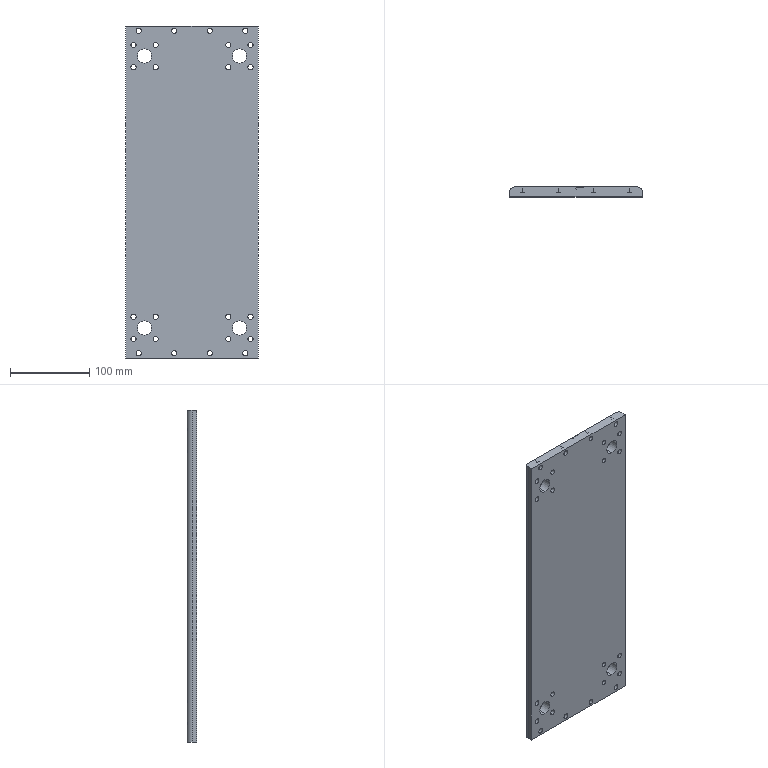Part | SolidWorks | features HoleWzd 2, ICE 2, MirrorPattern 2, Extrusion 1, Fillet 1, LPattern 1 | 1 solid | 309 faces | box 168 x 12 x 420 mm | volume 807216 mm3 | plane 203 | cylinder 106 | commonest cylinder face diameters 6.6 x48 11 x48 18 x8 12 x2